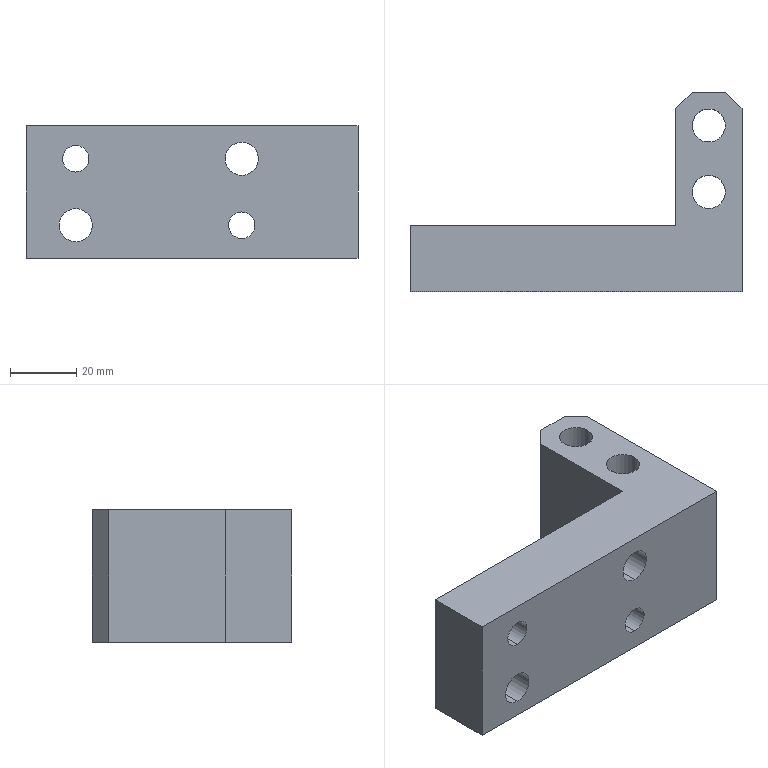Part | STEP file | HXGR200008-05-08 | 1 solid | 22 faces | box 100 x 60 x 40 mm | volume 99565 mm3 | cylinder 12 | plane 10 | commonest cylinder face diameters 10 x8 8 x4
STEP:
#1=CARTESIAN_POINT('',(-25.,0.,-14.));
#2=VERTEX_POINT('',#1);
#3=CARTESIAN_POINT('',(-25.,0.,-6.));
#4=VERTEX_POINT('',#3);
#5=CARTESIAN_POINT('',(-25.,0.,-10.));
#6=DIRECTION('',(0.,1.,0.));
#7=DIRECTION('',(0.,0.,1.));
#8=AXIS2_PLACEMENT_3D('',#5,#6,#7);
#9=CIRCLE('',#8,4.);
#10=EDGE_CURVE('',#2,#4,#9,.T.);
#11=ORIENTED_EDGE('',*,*,#10,.F.);
#12=CARTESIAN_POINT('',(-25.,20.,-14.));
#13=VERTEX_POINT('',#12);
#14=CARTESIAN_POINT('',(-25.,20.,-14.));
#15=DIRECTION('',(0.,1.,0.));
#16=VECTOR('',#15,1000.);
#17=LINE('',#14,#16);
#18=EDGE_CURVE('',#2,#13,#17,.T.);
#19=ORIENTED_EDGE('',*,*,#18,.T.);
#20=CARTESIAN_POINT('',(-25.,20.,-6.));
#21=VERTEX_POINT('',#20);
#22=CARTESIAN_POINT('',(-25.,20.,-10.));
#23=DIRECTION('',(0.,1.,0.));
#24=DIRECTION('',(0.,0.,1.));
#25=AXIS2_PLACEMENT_3D('',#22,#23,#24);
#26=CIRCLE('',#25,4.);
#27=EDGE_CURVE('',#13,#21,#26,.T.);
#28=ORIENTED_EDGE('',*,*,#27,.T.);
#29=CARTESIAN_POINT('',(-25.,20.,-6.));
#30=DIRECTION('',(0.,1.,0.));
#31=VECTOR('',#30,1000.);
#32=LINE('',#29,#31);
#33=EDGE_CURVE('',#4,#21,#32,.T.);
#34=ORIENTED_EDGE('',*,*,#33,.F.);
#35=EDGE_LOOP('',(#11,#19,#28,#34));
#36=FACE_OUTER_BOUND('',#35,.T.);
#37=CARTESIAN_POINT('',(-25.,20.,-10.));
#38=DIRECTION('',(0.,1.,0.));
#39=DIRECTION('',(0.,0.,1.));
#40=AXIS2_PLACEMENT_3D('',#37,#38,#39);
#41=CYLINDRICAL_SURFACE('',#40,4.);
#42=ADVANCED_FACE('',(#36),#41,.F.);
#43=CARTESIAN_POINT('',(-75.,0.,6.));
#44=VERTEX_POINT('',#43);
#45=CARTESIAN_POINT('',(-75.,0.,14.));
#46=VERTEX_POINT('',#45);
#47=CARTESIAN_POINT('',(-75.,0.,10.));
#48=DIRECTION('',(0.,1.,0.));
#49=DIRECTION('',(0.,0.,1.));
#50=AXIS2_PLACEMENT_3D('',#47,#48,#49);
#51=CIRCLE('',#50,4.);
#52=EDGE_CURVE('',#44,#46,#51,.T.);
#53=ORIENTED_EDGE('',*,*,#52,.F.);
#54=CARTESIAN_POINT('',(-75.,20.,6.));
#55=VERTEX_POINT('',#54);
#56=CARTESIAN_POINT('',(-75.,20.,6.));
#57=DIRECTION('',(0.,1.,0.));
#58=VECTOR('',#57,1000.);
#59=LINE('',#56,#58);
#60=EDGE_CURVE('',#44,#55,#59,.T.);
#61=ORIENTED_EDGE('',*,*,#60,.T.);
#62=CARTESIAN_POINT('',(-75.,20.,14.));
#63=VERTEX_POINT('',#62);
#64=CARTESIAN_POINT('',(-75.,20.,10.));
#65=DIRECTION('',(0.,1.,0.));
#66=DIRECTION('',(0.,0.,1.));
#67=AXIS2_PLACEMENT_3D('',#64,#65,#66);
#68=CIRCLE('',#67,4.);
#69=EDGE_CURVE('',#55,#63,#68,.T.);
#70=ORIENTED_EDGE('',*,*,#69,.T.);
#71=CARTESIAN_POINT('',(-75.,20.,14.));
#72=DIRECTION('',(0.,1.,0.));
#73=VECTOR('',#72,1000.);
#74=LINE('',#71,#73);
#75=EDGE_CURVE('',#46,#63,#74,.T.);
#76=ORIENTED_EDGE('',*,*,#75,.F.);
#77=EDGE_LOOP('',(#53,#61,#70,#76));
#78=FACE_OUTER_BOUND('',#77,.T.);
#79=CARTESIAN_POINT('',(-75.,20.,10.));
#80=DIRECTION('',(0.,1.,0.));
#81=DIRECTION('',(0.,0.,1.));
#82=AXIS2_PLACEMENT_3D('',#79,#80,#81);
#83=CYLINDRICAL_SURFACE('',#82,4.);
#84=ADVANCED_FACE('',(#78),#83,.F.);
#85=CARTESIAN_POINT('',(-75.,0.,-15.));
#86=VERTEX_POINT('',#85);
#87=CARTESIAN_POINT('',(-75.,0.,-5.));
#88=VERTEX_POINT('',#87);
#89=CARTESIAN_POINT('',(-75.,0.,-10.));
#90=DIRECTION('',(0.,1.,0.));
#91=DIRECTION('',(0.,0.,1.));
#92=AXIS2_PLACEMENT_3D('',#89,#90,#91);
#93=CIRCLE('',#92,5.);
#94=EDGE_CURVE('',#86,#88,#93,.T.);
#95=ORIENTED_EDGE('',*,*,#94,.F.);
#96=CARTESIAN_POINT('',(-75.,20.,-15.));
#97=VERTEX_POINT('',#96);
#98=CARTESIAN_POINT('',(-75.,20.,-15.));
#99=DIRECTION('',(0.,1.,0.));
#100=VECTOR('',#99,1000.);
#101=LINE('',#98,#100);
#102=EDGE_CURVE('',#86,#97,#101,.T.);
#103=ORIENTED_EDGE('',*,*,#102,.T.);
#104=CARTESIAN_POINT('',(-75.,20.,-5.));
#105=VERTEX_POINT('',#104);
#106=CARTESIAN_POINT('',(-75.,20.,-10.));
#107=DIRECTION('',(0.,1.,0.));
#108=DIRECTION('',(0.,0.,1.));
#109=AXIS2_PLACEMENT_3D('',#106,#107,#108);
#110=CIRCLE('',#109,5.);
#111=EDGE_CURVE('',#97,#105,#110,.T.);
#112=ORIENTED_EDGE('',*,*,#111,.T.);
#113=CARTESIAN_POINT('',(-75.,20.,-5.));
#114=DIRECTION('',(0.,1.,0.));
#115=VECTOR('',#114,1000.);
#116=LINE('',#113,#115);
#117=EDGE_CURVE('',#88,#105,#116,.T.);
#118=ORIENTED_EDGE('',*,*,#117,.F.);
#119=EDGE_LOOP('',(#95,#103,#112,#118));
#120=FACE_OUTER_BOUND('',#119,.T.);
#121=CARTESIAN_POINT('',(-75.,20.,-10.));
#122=DIRECTION('',(0.,1.,0.));
#123=DIRECTION('',(0.,0.,1.));
#124=AXIS2_PLACEMENT_3D('',#121,#122,#123);
#125=CYLINDRICAL_SURFACE('',#124,5.);
#126=ADVANCED_FACE('',(#120),#125,.F.);
#127=CARTESIAN_POINT('',(-25.,0.,5.));
#128=VERTEX_POINT('',#127);
#129=CARTESIAN_POINT('',(-25.,0.,15.));
#130=VERTEX_POINT('',#129);
#131=CARTESIAN_POINT('',(-25.,0.,10.));
#132=DIRECTION('',(0.,1.,0.));
#133=DIRECTION('',(0.,0.,1.));
#134=AXIS2_PLACEMENT_3D('',#131,#132,#133);
#135=CIRCLE('',#134,5.);
#136=EDGE_CURVE('',#128,#130,#135,.T.);
#137=ORIENTED_EDGE('',*,*,#136,.F.);
#138=CARTESIAN_POINT('',(-25.,20.,5.));
#139=VERTEX_POINT('',#138);
#140=CARTESIAN_POINT('',(-25.,20.,5.));
#141=DIRECTION('',(0.,1.,0.));
#142=VECTOR('',#141,1000.);
#143=LINE('',#140,#142);
#144=EDGE_CURVE('',#128,#139,#143,.T.);
#145=ORIENTED_EDGE('',*,*,#144,.T.);
#146=CARTESIAN_POINT('',(-25.,20.,15.));
#147=VERTEX_POINT('',#146);
#148=CARTESIAN_POINT('',(-25.,20.,10.));
#149=DIRECTION('',(0.,1.,0.));
#150=DIRECTION('',(0.,0.,1.));
#151=AXIS2_PLACEMENT_3D('',#148,#149,#150);
#152=CIRCLE('',#151,5.);
#153=EDGE_CURVE('',#139,#147,#152,.T.);
#154=ORIENTED_EDGE('',*,*,#153,.T.);
#155=CARTESIAN_POINT('',(-25.,20.,15.));
#156=DIRECTION('',(0.,1.,0.));
#157=VECTOR('',#156,1000.);
#158=LINE('',#155,#157);
#159=EDGE_CURVE('',#130,#147,#158,.T.);
#160=ORIENTED_EDGE('',*,*,#159,.F.);
#161=EDGE_LOOP('',(#137,#145,#154,#160));
#162=FACE_OUTER_BOUND('',#161,.T.);
#163=CARTESIAN_POINT('',(-25.,20.,10.));
#164=DIRECTION('',(0.,1.,0.));
#165=DIRECTION('',(0.,0.,1.));
#166=AXIS2_PLACEMENT_3D('',#163,#164,#165);
#167=CYLINDRICAL_SURFACE('',#166,5.);
#168=ADVANCED_FACE('',(#162),#167,.F.);
#169=CARTESIAN_POINT('',(-5.,50.,-20.));
#170=VERTEX_POINT('',#169);
#171=CARTESIAN_POINT('',(5.,50.,-20.));
#172=VERTEX_POINT('',#171);
#173=CARTESIAN_POINT('',(0.,50.,-20.));
#174=DIRECTION('',(0.,0.,1.));
#175=DIRECTION('',(1.,0.,0.));
#176=AXIS2_PLACEMENT_3D('',#173,#174,#175);
#177=CIRCLE('',#176,5.);
#178=EDGE_CURVE('',#170,#172,#177,.T.);
#179=ORIENTED_EDGE('',*,*,#178,.F.);
#180=CARTESIAN_POINT('',(-5.,50.,20.));
#181=VERTEX_POINT('',#180);
#182=CARTESIAN_POINT('',(-5.,50.,20.));
#183=DIRECTION('',(0.,0.,1.));
#184=VECTOR('',#183,1000.);
#185=LINE('',#182,#184);
#186=EDGE_CURVE('',#170,#181,#185,.T.);
#187=ORIENTED_EDGE('',*,*,#186,.T.);
#188=CARTESIAN_POINT('',(5.,50.,20.));
#189=VERTEX_POINT('',#188);
#190=CARTESIAN_POINT('',(0.,50.,20.));
#191=DIRECTION('',(0.,0.,1.));
#192=DIRECTION('',(1.,0.,0.));
#193=AXIS2_PLACEMENT_3D('',#190,#191,#192);
#194=CIRCLE('',#193,5.);
#195=EDGE_CURVE('',#181,#189,#194,.T.);
#196=ORIENTED_EDGE('',*,*,#195,.T.);
#197=CARTESIAN_POINT('',(5.,50.,20.));
#198=DIRECTION('',(0.,0.,1.));
#199=VECTOR('',#198,1000.);
#200=LINE('',#197,#199);
#201=EDGE_CURVE('',#172,#189,#200,.T.);
#202=ORIENTED_EDGE('',*,*,#201,.F.);
#203=EDGE_LOOP('',(#179,#187,#196,#202));
#204=FACE_OUTER_BOUND('',#203,.T.);
#205=CARTESIAN_POINT('',(0.,50.,20.));
#206=DIRECTION('',(0.,0.,1.));
#207=DIRECTION('',(1.,0.,0.));
#208=AXIS2_PLACEMENT_3D('',#205,#206,#207);
#209=CYLINDRICAL_SURFACE('',#208,5.);
#210=ADVANCED_FACE('',(#204),#209,.F.);
#211=CARTESIAN_POINT('',(-5.,30.,-20.));
#212=VERTEX_POINT('',#211);
#213=CARTESIAN_POINT('',(5.,30.,-20.));
#214=VERTEX_POINT('',#213);
#215=CARTESIAN_POINT('',(0.,30.,-20.));
#216=DIRECTION('',(0.,0.,1.));
#217=DIRECTION('',(1.,0.,0.));
#218=AXIS2_PLACEMENT_3D('',#215,#216,#217);
#219=CIRCLE('',#218,5.);
#220=EDGE_CURVE('',#212,#214,#219,.T.);
#221=ORIENTED_EDGE('',*,*,#220,.F.);
#222=CARTESIAN_POINT('',(-5.,30.,20.));
#223=VERTEX_POINT('',#222);
#224=CARTESIAN_POINT('',(-5.,30.,20.));
#225=DIRECTION('',(0.,0.,1.));
#226=VECTOR('',#225,1000.);
#227=LINE('',#224,#226);
#228=EDGE_CURVE('',#212,#223,#227,.T.);
#229=ORIENTED_EDGE('',*,*,#228,.T.);
#230=CARTESIAN_POINT('',(5.,30.,20.));
#231=VERTEX_POINT('',#230);
#232=CARTESIAN_POINT('',(0.,30.,20.));
#233=DIRECTION('',(0.,0.,1.));
#234=DIRECTION('',(1.,0.,0.));
#235=AXIS2_PLACEMENT_3D('',#232,#233,#234);
#236=CIRCLE('',#235,5.);
#237=EDGE_CURVE('',#223,#231,#236,.T.);
#238=ORIENTED_EDGE('',*,*,#237,.T.);
#239=CARTESIAN_POINT('',(5.,30.,20.));
#240=DIRECTION('',(0.,0.,1.));
#241=VECTOR('',#240,1000.);
#242=LINE('',#239,#241);
#243=EDGE_CURVE('',#214,#231,#242,.T.);
#244=ORIENTED_EDGE('',*,*,#243,.F.);
#245=EDGE_LOOP('',(#221,#229,#238,#244));
#246=FACE_OUTER_BOUND('',#245,.T.);
#247=CARTESIAN_POINT('',(0.,30.,20.));
#248=DIRECTION('',(0.,0.,1.));
#249=DIRECTION('',(1.,0.,0.));
#250=AXIS2_PLACEMENT_3D('',#247,#248,#249);
#251=CYLINDRICAL_SURFACE('',#250,5.);
#252=ADVANCED_FACE('',(#246),#251,.F.);
#253=CARTESIAN_POINT('',(10.,0.,-20.));
#254=VERTEX_POINT('',#253);
#255=CARTESIAN_POINT('',(10.,55.,-20.));
#256=VERTEX_POINT('',#255);
#257=CARTESIAN_POINT('',(10.,60.,-20.));
#258=DIRECTION('',(0.,1.,0.));
#259=VECTOR('',#258,1000.);
#260=LINE('',#257,#259);
#261=EDGE_CURVE('',#254,#256,#260,.T.);
#262=ORIENTED_EDGE('',*,*,#261,.T.);
#263=CARTESIAN_POINT('',(10.,55.,20.));
#264=VERTEX_POINT('',#263);
#265=CARTESIAN_POINT('',(10.,55.,20.));
#266=DIRECTION('',(0.,0.,1.));
#267=VECTOR('',#266,1000.);
#268=LINE('',#265,#267);
#269=EDGE_CURVE('',#256,#264,#268,.T.);
#270=ORIENTED_EDGE('',*,*,#269,.T.);
#271=CARTESIAN_POINT('',(10.,0.,20.));
#272=VERTEX_POINT('',#271);
#273=CARTESIAN_POINT('',(10.,60.,20.));
#274=DIRECTION('',(0.,1.,0.));
#275=VECTOR('',#274,1000.);
#276=LINE('',#273,#275);
#277=EDGE_CURVE('',#272,#264,#276,.T.);
#278=ORIENTED_EDGE('',*,*,#277,.F.);
#279=CARTESIAN_POINT('',(10.,0.,20.));
#280=DIRECTION('',(0.,0.,-1.));
#281=VECTOR('',#280,1000.);
#282=LINE('',#279,#281);
#283=EDGE_CURVE('',#272,#254,#282,.T.);
#284=ORIENTED_EDGE('',*,*,#283,.T.);
#285=EDGE_LOOP('',(#262,#270,#278,#284));
#286=FACE_OUTER_BOUND('',#285,.T.);
#287=CARTESIAN_POINT('',(10.,60.,20.));
#288=DIRECTION('',(-1.,0.,0.));
#289=DIRECTION('',(0.,-1.,0.));
#290=AXIS2_PLACEMENT_3D('',#287,#288,#289);
#291=PLANE('',#290);
#292=ADVANCED_FACE('',(#286),#291,.F.);
#293=CARTESIAN_POINT('',(5.,60.,20.));
#294=VERTEX_POINT('',#293);
#295=CARTESIAN_POINT('',(-5.,60.,20.));
#296=VERTEX_POINT('',#295);
#297=CARTESIAN_POINT('',(-10.,60.,20.));
#298=DIRECTION('',(-1.,0.,0.));
#299=VECTOR('',#298,1000.);
#300=LINE('',#297,#299);
#301=EDGE_CURVE('',#294,#296,#300,.T.);
#302=ORIENTED_EDGE('',*,*,#301,.F.);
#303=CARTESIAN_POINT('',(5.,60.,-20.));
#304=VERTEX_POINT('',#303);
#305=CARTESIAN_POINT('',(5.,60.,20.));
#306=DIRECTION('',(0.,0.,-1.));
#307=VECTOR('',#306,1000.);
#308=LINE('',#305,#307);
#309=EDGE_CURVE('',#294,#304,#308,.T.);
#310=ORIENTED_EDGE('',*,*,#309,.T.);
#311=CARTESIAN_POINT('',(-5.,60.,-20.));
#312=VERTEX_POINT('',#311);
#313=CARTESIAN_POINT('',(-10.,60.,-20.));
#314=DIRECTION('',(-1.,0.,0.));
#315=VECTOR('',#314,1000.);
#316=LINE('',#313,#315);
#317=EDGE_CURVE('',#304,#312,#316,.T.);
#318=ORIENTED_EDGE('',*,*,#317,.T.);
#319=CARTESIAN_POINT('',(-5.,60.,20.));
#320=DIRECTION('',(0.,0.,1.));
#321=VECTOR('',#320,1000.);
#322=LINE('',#319,#321);
#323=EDGE_CURVE('',#312,#296,#322,.T.);
#324=ORIENTED_EDGE('',*,*,#323,.T.);
#325=EDGE_LOOP('',(#302,#310,#318,#324));
#326=FACE_OUTER_BOUND('',#325,.T.);
#327=CARTESIAN_POINT('',(-10.,60.,20.));
#328=DIRECTION('',(0.,-1.,0.));
#329=DIRECTION('',(1.,0.,0.));
#330=AXIS2_PLACEMENT_3D('',#327,#328,#329);
#331=PLANE('',#330);
#332=ADVANCED_FACE('',(#326),#331,.F.);
#333=CARTESIAN_POINT('',(-10.,55.,20.));
#334=VERTEX_POINT('',#333);
#335=CARTESIAN_POINT('',(-10.,20.,20.));
#336=VERTEX_POINT('',#335);
#337=CARTESIAN_POINT('',(-10.,60.,20.));
#338=DIRECTION('',(0.,-1.,0.));
#339=VECTOR('',#338,1000.);
#340=LINE('',#337,#339);
#341=EDGE_CURVE('',#334,#336,#340,.T.);
#342=ORIENTED_EDGE('',*,*,#341,.F.);
#343=CARTESIAN_POINT('',(-10.,55.,-20.));
#344=VERTEX_POINT('',#343);
#345=CARTESIAN_POINT('',(-10.,55.,20.));
#346=DIRECTION('',(0.,0.,-1.));
#347=VECTOR('',#346,1000.);
#348=LINE('',#345,#347);
#349=EDGE_CURVE('',#334,#344,#348,.T.);
#350=ORIENTED_EDGE('',*,*,#349,.T.);
#351=CARTESIAN_POINT('',(-10.,20.,-20.));
#352=VERTEX_POINT('',#351);
#353=CARTESIAN_POINT('',(-10.,60.,-20.));
#354=DIRECTION('',(0.,-1.,0.));
#355=VECTOR('',#354,1000.);
#356=LINE('',#353,#355);
#357=EDGE_CURVE('',#344,#352,#356,.T.);
#358=ORIENTED_EDGE('',*,*,#357,.T.);
#359=CARTESIAN_POINT('',(-10.,20.,20.));
#360=DIRECTION('',(0.,0.,-1.));
#361=VECTOR('',#360,1000.);
#362=LINE('',#359,#361);
#363=EDGE_CURVE('',#336,#352,#362,.T.);
#364=ORIENTED_EDGE('',*,*,#363,.F.);
#365=EDGE_LOOP('',(#342,#350,#358,#364));
#366=FACE_OUTER_BOUND('',#365,.T.);
#367=CARTESIAN_POINT('',(-10.,60.,20.));
#368=DIRECTION('',(1.,0.,0.));
#369=DIRECTION('',(0.,1.,0.));
#370=AXIS2_PLACEMENT_3D('',#367,#368,#369);
#371=PLANE('',#370);
#372=ADVANCED_FACE('',(#366),#371,.F.);
#373=CARTESIAN_POINT('',(-25.,20.,-10.));
#374=DIRECTION('',(0.,1.,0.));
#375=DIRECTION('',(0.,0.,1.));
#376=AXIS2_PLACEMENT_3D('',#373,#374,#375);
#377=CIRCLE('',#376,4.);
#378=EDGE_CURVE('',#21,#13,#377,.T.);
#379=ORIENTED_EDGE('',*,*,#378,.F.);
#380=ORIENTED_EDGE('',*,*,#27,.F.);
#381=EDGE_LOOP('',(#379,#380));
#382=FACE_BOUND('',#381,.T.);
#383=CARTESIAN_POINT('',(-75.,20.,10.));
#384=DIRECTION('',(0.,1.,0.));
#385=DIRECTION('',(0.,0.,1.));
#386=AXIS2_PLACEMENT_3D('',#383,#384,#385);
#387=CIRCLE('',#386,4.);
#388=EDGE_CURVE('',#63,#55,#387,.T.);
#389=ORIENTED_EDGE('',*,*,#388,.F.);
#390=ORIENTED_EDGE('',*,*,#69,.F.);
#391=EDGE_LOOP('',(#389,#390));
#392=FACE_BOUND('',#391,.T.);
#393=CARTESIAN_POINT('',(-75.,20.,-10.));
#394=DIRECTION('',(0.,1.,0.));
#395=DIRECTION('',(0.,0.,1.));
#396=AXIS2_PLACEMENT_3D('',#393,#394,#395);
#397=CIRCLE('',#396,5.);
#398=EDGE_CURVE('',#105,#97,#397,.T.);
#399=ORIENTED_EDGE('',*,*,#398,.F.);
#400=ORIENTED_EDGE('',*,*,#111,.F.);
#401=EDGE_LOOP('',(#399,#400));
#402=FACE_BOUND('',#401,.T.);
#403=CARTESIAN_POINT('',(-25.,20.,10.));
#404=DIRECTION('',(0.,1.,0.));
#405=DIRECTION('',(0.,0.,1.));
#406=AXIS2_PLACEMENT_3D('',#403,#404,#405);
#407=CIRCLE('',#406,5.);
#408=EDGE_CURVE('',#147,#139,#407,.T.);
#409=ORIENTED_EDGE('',*,*,#408,.F.);
#410=ORIENTED_EDGE('',*,*,#153,.F.);
#411=EDGE_LOOP('',(#409,#410));
#412=FACE_BOUND('',#411,.T.);
#413=CARTESIAN_POINT('',(-90.,20.,-20.));
#414=VERTEX_POINT('',#413);
#415=CARTESIAN_POINT('',(-90.,20.,-20.));
#416=DIRECTION('',(-1.,0.,0.));
#417=VECTOR('',#416,1000.);
#418=LINE('',#415,#417);
#419=EDGE_CURVE('',#352,#414,#418,.T.);
#420=ORIENTED_EDGE('',*,*,#419,.T.);
#421=CARTESIAN_POINT('',(-90.,20.,20.));
#422=VERTEX_POINT('',#421);
#423=CARTESIAN_POINT('',(-90.,20.,20.));
#424=DIRECTION('',(0.,0.,-1.));
#425=VECTOR('',#424,1000.);
#426=LINE('',#423,#425);
#427=EDGE_CURVE('',#422,#414,#426,.T.);
#428=ORIENTED_EDGE('',*,*,#427,.F.);
#429=CARTESIAN_POINT('',(-90.,20.,20.));
#430=DIRECTION('',(-1.,0.,0.));
#431=VECTOR('',#430,1000.);
#432=LINE('',#429,#431);
#433=EDGE_CURVE('',#336,#422,#432,.T.);
#434=ORIENTED_EDGE('',*,*,#433,.F.);
#435=ORIENTED_EDGE('',*,*,#363,.T.);
#436=EDGE_LOOP('',(#420,#428,#434,#435));
#437=FACE_OUTER_BOUND('',#436,.T.);
#438=CARTESIAN_POINT('',(-90.,20.,20.));
#439=DIRECTION('',(0.,-1.,0.));
#440=DIRECTION('',(0.,0.,-1.));
#441=AXIS2_PLACEMENT_3D('',#438,#439,#440);
#442=PLANE('',#441);
#443=ADVANCED_FACE('',(#382,#392,#402,#412,#437),#442,.F.);
#444=CARTESIAN_POINT('',(-90.,0.,-20.));
#445=VERTEX_POINT('',#444);
#446=CARTESIAN_POINT('',(-90.,20.,-20.));
#447=DIRECTION('',(0.,-1.,0.));
#448=VECTOR('',#447,1000.);
#449=LINE('',#446,#448);
#450=EDGE_CURVE('',#414,#445,#449,.T.);
#451=ORIENTED_EDGE('',*,*,#450,.T.);
#452=CARTESIAN_POINT('',(-90.,0.,20.));
#453=VERTEX_POINT('',#452);
#454=CARTESIAN_POINT('',(-90.,0.,20.));
#455=DIRECTION('',(0.,0.,-1.));
#456=VECTOR('',#455,1000.);
#457=LINE('',#454,#456);
#458=EDGE_CURVE('',#453,#445,#457,.T.);
#459=ORIENTED_EDGE('',*,*,#458,.F.);
#460=CARTESIAN_POINT('',(-90.,20.,20.));
#461=DIRECTION('',(0.,-1.,0.));
#462=VECTOR('',#461,1000.);
#463=LINE('',#460,#462);
#464=EDGE_CURVE('',#422,#453,#463,.T.);
#465=ORIENTED_EDGE('',*,*,#464,.F.);
#466=ORIENTED_EDGE('',*,*,#427,.T.);
#467=EDGE_LOOP('',(#451,#459,#465,#466));
#468=FACE_OUTER_BOUND('',#467,.T.);
#469=CARTESIAN_POINT('',(-90.,20.,20.));
#470=DIRECTION('',(1.,0.,0.));
#471=DIRECTION('',(0.,1.,0.));
#472=AXIS2_PLACEMENT_3D('',#469,#470,#471);
#473=PLANE('',#472);
#474=ADVANCED_FACE('',(#468),#473,.F.);
#475=CARTESIAN_POINT('',(-25.,0.,-10.));
#476=DIRECTION('',(0.,1.,0.));
#477=DIRECTION('',(0.,0.,1.));
#478=AXIS2_PLACEMENT_3D('',#475,#476,#477);
#479=CIRCLE('',#478,4.);
#480=EDGE_CURVE('',#4,#2,#479,.T.);
#481=ORIENTED_EDGE('',*,*,#480,.T.);
#482=ORIENTED_EDGE('',*,*,#10,.T.);
#483=EDGE_LOOP('',(#481,#482));
#484=FACE_BOUND('',#483,.T.);
#485=CARTESIAN_POINT('',(-75.,0.,10.));
#486=DIRECTION('',(0.,1.,0.));
#487=DIRECTION('',(0.,0.,1.));
#488=AXIS2_PLACEMENT_3D('',#485,#486,#487);
#489=CIRCLE('',#488,4.);
#490=EDGE_CURVE('',#46,#44,#489,.T.);
#491=ORIENTED_EDGE('',*,*,#490,.T.);
#492=ORIENTED_EDGE('',*,*,#52,.T.);
#493=EDGE_LOOP('',(#491,#492));
#494=FACE_BOUND('',#493,.T.);
#495=CARTESIAN_POINT('',(-75.,0.,-10.));
#496=DIRECTION('',(0.,1.,0.));
#497=DIRECTION('',(0.,0.,1.));
#498=AXIS2_PLACEMENT_3D('',#495,#496,#497);
#499=CIRCLE('',#498,5.);
#500=EDGE_CURVE('',#88,#86,#499,.T.);
#501=ORIENTED_EDGE('',*,*,#500,.T.);
#502=ORIENTED_EDGE('',*,*,#94,.T.);
#503=EDGE_LOOP('',(#501,#502));
#504=FACE_BOUND('',#503,.T.);
#505=CARTESIAN_POINT('',(-25.,0.,10.));
#506=DIRECTION('',(0.,1.,0.));
#507=DIRECTION('',(0.,0.,1.));
#508=AXIS2_PLACEMENT_3D('',#505,#506,#507);
#509=CIRCLE('',#508,5.);
#510=EDGE_CURVE('',#130,#128,#509,.T.);
#511=ORIENTED_EDGE('',*,*,#510,.T.);
#512=ORIENTED_EDGE('',*,*,#136,.T.);
#513=EDGE_LOOP('',(#511,#512));
#514=FACE_BOUND('',#513,.T.);
#515=CARTESIAN_POINT('',(10.,0.,-20.));
#516=DIRECTION('',(1.,0.,0.));
#517=VECTOR('',#516,1000.);
#518=LINE('',#515,#517);
#519=EDGE_CURVE('',#445,#254,#518,.T.);
#520=ORIENTED_EDGE('',*,*,#519,.T.);
#521=ORIENTED_EDGE('',*,*,#283,.F.);
#522=CARTESIAN_POINT('',(10.,0.,20.));
#523=DIRECTION('',(1.,0.,0.));
#524=VECTOR('',#523,1000.);
#525=LINE('',#522,#524);
#526=EDGE_CURVE('',#453,#272,#525,.T.);
#527=ORIENTED_EDGE('',*,*,#526,.F.);
#528=ORIENTED_EDGE('',*,*,#458,.T.);
#529=EDGE_LOOP('',(#520,#521,#527,#528));
#530=FACE_OUTER_BOUND('',#529,.T.);
#531=CARTESIAN_POINT('',(10.,0.,20.));
#532=DIRECTION('',(0.,1.,0.));
#533=DIRECTION('',(-1.,0.,0.));
#534=AXIS2_PLACEMENT_3D('',#531,#532,#533);
#535=PLANE('',#534);
#536=ADVANCED_FACE('',(#484,#494,#504,#514,#530),#535,.F.);
#537=CARTESIAN_POINT('',(0.,50.,20.));
#538=DIRECTION('',(0.,0.,1.));
#539=DIRECTION('',(1.,0.,0.));
#540=AXIS2_PLACEMENT_3D('',#537,#538,#539);
#541=CIRCLE('',#540,5.);
#542=EDGE_CURVE('',#189,#181,#541,.T.);
#543=ORIENTED_EDGE('',*,*,#542,.F.);
#544=ORIENTED_EDGE('',*,*,#195,.F.);
#545=EDGE_LOOP('',(#543,#544));
#546=FACE_BOUND('',#545,.T.);
#547=CARTESIAN_POINT('',(0.,30.,20.));
#548=DIRECTION('',(0.,0.,1.));
#549=DIRECTION('',(1.,0.,0.));
#550=AXIS2_PLACEMENT_3D('',#547,#548,#549);
#551=CIRCLE('',#550,5.);
#552=EDGE_CURVE('',#231,#223,#551,.T.);
#553=ORIENTED_EDGE('',*,*,#552,.F.);
#554=ORIENTED_EDGE('',*,*,#237,.F.);
#555=EDGE_LOOP('',(#553,#554));
#556=FACE_BOUND('',#555,.T.);
#557=ORIENTED_EDGE('',*,*,#277,.T.);
#558=CARTESIAN_POINT('',(5.,60.,20.));
#559=DIRECTION('',(-0.7071,0.7071,0.));
#560=VECTOR('',#559,1000.);
#561=LINE('',#558,#560);
#562=EDGE_CURVE('',#264,#294,#561,.T.);
#563=ORIENTED_EDGE('',*,*,#562,.T.);
#564=ORIENTED_EDGE('',*,*,#301,.T.);
#565=CARTESIAN_POINT('',(-10.,55.,20.));
#566=DIRECTION('',(-0.7071,-0.7071,0.));
#567=VECTOR('',#566,1000.);
#568=LINE('',#565,#567);
#569=EDGE_CURVE('',#296,#334,#568,.T.);
#570=ORIENTED_EDGE('',*,*,#569,.T.);
#571=ORIENTED_EDGE('',*,*,#341,.T.);
#572=ORIENTED_EDGE('',*,*,#433,.T.);
#573=ORIENTED_EDGE('',*,*,#464,.T.);
#574=ORIENTED_EDGE('',*,*,#526,.T.);
#575=EDGE_LOOP('',(#557,#563,#564,#570,#571,#572,#573,#574));
#576=FACE_OUTER_BOUND('',#575,.T.);
#577=CARTESIAN_POINT('',(0.,0.,20.));
#578=DIRECTION('',(0.,0.,-1.));
#579=DIRECTION('',(-1.,0.,0.));
#580=AXIS2_PLACEMENT_3D('',#577,#578,#579);
#581=PLANE('',#580);
#582=ADVANCED_FACE('',(#546,#556,#576),#581,.F.);
#583=CARTESIAN_POINT('',(0.,50.,-20.));
#584=DIRECTION('',(0.,0.,1.));
#585=DIRECTION('',(1.,0.,0.));
#586=AXIS2_PLACEMENT_3D('',#583,#584,#585);
#587=CIRCLE('',#586,5.);
#588=EDGE_CURVE('',#172,#170,#587,.T.);
#589=ORIENTED_EDGE('',*,*,#588,.T.);
#590=ORIENTED_EDGE('',*,*,#178,.T.);
#591=EDGE_LOOP('',(#589,#590));
#592=FACE_BOUND('',#591,.T.);
#593=CARTESIAN_POINT('',(0.,30.,-20.));
#594=DIRECTION('',(0.,0.,1.));
#595=DIRECTION('',(1.,0.,0.));
#596=AXIS2_PLACEMENT_3D('',#593,#594,#595);
#597=CIRCLE('',#596,5.);
#598=EDGE_CURVE('',#214,#212,#597,.T.);
#599=ORIENTED_EDGE('',*,*,#598,.T.);
#600=ORIENTED_EDGE('',*,*,#220,.T.);
#601=EDGE_LOOP('',(#599,#600));
#602=FACE_BOUND('',#601,.T.);
#603=ORIENTED_EDGE('',*,*,#317,.F.);
#604=CARTESIAN_POINT('',(32.5,32.5,-20.));
#605=DIRECTION('',(0.7071,-0.7071,0.));
#606=VECTOR('',#605,1000.);
#607=LINE('',#604,#606);
#608=EDGE_CURVE('',#304,#256,#607,.T.);
#609=ORIENTED_EDGE('',*,*,#608,.T.);
#610=ORIENTED_EDGE('',*,*,#261,.F.);
#611=ORIENTED_EDGE('',*,*,#519,.F.);
#612=ORIENTED_EDGE('',*,*,#450,.F.);
#613=ORIENTED_EDGE('',*,*,#419,.F.);
#614=ORIENTED_EDGE('',*,*,#357,.F.);
#615=CARTESIAN_POINT('',(-32.5,32.5,-20.));
#616=DIRECTION('',(0.7071,0.7071,0.));
#617=VECTOR('',#616,1000.);
#618=LINE('',#615,#617);
#619=EDGE_CURVE('',#344,#312,#618,.T.);
#620=ORIENTED_EDGE('',*,*,#619,.T.);
#621=EDGE_LOOP('',(#603,#609,#610,#611,#612,#613,#614,#620));
#622=FACE_OUTER_BOUND('',#621,.T.);
#623=CARTESIAN_POINT('',(0.,0.,-20.));
#624=DIRECTION('',(0.,0.,-1.));
#625=DIRECTION('',(-1.,0.,0.));
#626=AXIS2_PLACEMENT_3D('',#623,#624,#625);
#627=PLANE('',#626);
#628=ADVANCED_FACE('',(#592,#602,#622),#627,.T.);
#629=ORIENTED_EDGE('',*,*,#228,.F.);
#630=ORIENTED_EDGE('',*,*,#598,.F.);
#631=ORIENTED_EDGE('',*,*,#243,.T.);
#632=ORIENTED_EDGE('',*,*,#552,.T.);
#633=EDGE_LOOP('',(#629,#630,#631,#632));
#634=FACE_OUTER_BOUND('',#633,.T.);
#635=CARTESIAN_POINT('',(0.,30.,20.));
#636=DIRECTION('',(0.,0.,1.));
#637=DIRECTION('',(1.,0.,0.));
#638=AXIS2_PLACEMENT_3D('',#635,#636,#637);
#639=CYLINDRICAL_SURFACE('',#638,5.);
#640=ADVANCED_FACE('',(#634),#639,.F.);
#641=ORIENTED_EDGE('',*,*,#186,.F.);
#642=ORIENTED_EDGE('',*,*,#588,.F.);
#643=ORIENTED_EDGE('',*,*,#201,.T.);
#644=ORIENTED_EDGE('',*,*,#542,.T.);
#645=EDGE_LOOP('',(#641,#642,#643,#644));
#646=FACE_OUTER_BOUND('',#645,.T.);
#647=CARTESIAN_POINT('',(0.,50.,20.));
#648=DIRECTION('',(0.,0.,1.));
#649=DIRECTION('',(1.,0.,0.));
#650=AXIS2_PLACEMENT_3D('',#647,#648,#649);
#651=CYLINDRICAL_SURFACE('',#650,5.);
#652=ADVANCED_FACE('',(#646),#651,.F.);
#653=ORIENTED_EDGE('',*,*,#562,.F.);
#654=ORIENTED_EDGE('',*,*,#269,.F.);
#655=ORIENTED_EDGE('',*,*,#608,.F.);
#656=ORIENTED_EDGE('',*,*,#309,.F.);
#657=EDGE_LOOP('',(#653,#654,#655,#656));
#658=FACE_OUTER_BOUND('',#657,.T.);
#659=CARTESIAN_POINT('',(5.,60.,20.));
#660=DIRECTION('',(-0.7071,-0.7071,0.));
#661=DIRECTION('',(0.,0.,-1.));
#662=AXIS2_PLACEMENT_3D('',#659,#660,#661);
#663=PLANE('',#662);
#664=ADVANCED_FACE('',(#658),#663,.F.);
#665=ORIENTED_EDGE('',*,*,#569,.F.);
#666=ORIENTED_EDGE('',*,*,#323,.F.);
#667=ORIENTED_EDGE('',*,*,#619,.F.);
#668=ORIENTED_EDGE('',*,*,#349,.F.);
#669=EDGE_LOOP('',(#665,#666,#667,#668));
#670=FACE_OUTER_BOUND('',#669,.T.);
#671=CARTESIAN_POINT('',(-10.,55.,20.));
#672=DIRECTION('',(0.7071,-0.7071,0.));
#673=DIRECTION('',(0.,0.,-1.));
#674=AXIS2_PLACEMENT_3D('',#671,#672,#673);
#675=PLANE('',#674);
#676=ADVANCED_FACE('',(#670),#675,.F.);
#677=ORIENTED_EDGE('',*,*,#144,.F.);
#678=ORIENTED_EDGE('',*,*,#510,.F.);
#679=ORIENTED_EDGE('',*,*,#159,.T.);
#680=ORIENTED_EDGE('',*,*,#408,.T.);
#681=EDGE_LOOP('',(#677,#678,#679,#680));
#682=FACE_OUTER_BOUND('',#681,.T.);
#683=CARTESIAN_POINT('',(-25.,20.,10.));
#684=DIRECTION('',(0.,1.,0.));
#685=DIRECTION('',(0.,0.,1.));
#686=AXIS2_PLACEMENT_3D('',#683,#684,#685);
#687=CYLINDRICAL_SURFACE('',#686,5.);
#688=ADVANCED_FACE('',(#682),#687,.F.);
#689=ORIENTED_EDGE('',*,*,#102,.F.);
#690=ORIENTED_EDGE('',*,*,#500,.F.);
#691=ORIENTED_EDGE('',*,*,#117,.T.);
#692=ORIENTED_EDGE('',*,*,#398,.T.);
#693=EDGE_LOOP('',(#689,#690,#691,#692));
#694=FACE_OUTER_BOUND('',#693,.T.);
#695=CARTESIAN_POINT('',(-75.,20.,-10.));
#696=DIRECTION('',(0.,1.,0.));
#697=DIRECTION('',(0.,0.,1.));
#698=AXIS2_PLACEMENT_3D('',#695,#696,#697);
#699=CYLINDRICAL_SURFACE('',#698,5.);
#700=ADVANCED_FACE('',(#694),#699,.F.);
#701=ORIENTED_EDGE('',*,*,#60,.F.);
#702=ORIENTED_EDGE('',*,*,#490,.F.);
#703=ORIENTED_EDGE('',*,*,#75,.T.);
#704=ORIENTED_EDGE('',*,*,#388,.T.);
#705=EDGE_LOOP('',(#701,#702,#703,#704));
#706=FACE_OUTER_BOUND('',#705,.T.);
#707=CARTESIAN_POINT('',(-75.,20.,10.));
#708=DIRECTION('',(0.,1.,0.));
#709=DIRECTION('',(0.,0.,1.));
#710=AXIS2_PLACEMENT_3D('',#707,#708,#709);
#711=CYLINDRICAL_SURFACE('',#710,4.);
#712=ADVANCED_FACE('',(#706),#711,.F.);
#713=ORIENTED_EDGE('',*,*,#18,.F.);
#714=ORIENTED_EDGE('',*,*,#480,.F.);
#715=ORIENTED_EDGE('',*,*,#33,.T.);
#716=ORIENTED_EDGE('',*,*,#378,.T.);
#717=EDGE_LOOP('',(#713,#714,#715,#716));
#718=FACE_OUTER_BOUND('',#717,.T.);
#719=CARTESIAN_POINT('',(-25.,20.,-10.));
#720=DIRECTION('',(0.,1.,0.));
#721=DIRECTION('',(0.,0.,1.));
#722=AXIS2_PLACEMENT_3D('',#719,#720,#721);
#723=CYLINDRICAL_SURFACE('',#722,4.);
#724=ADVANCED_FACE('',(#718),#723,.F.);
#725=CLOSED_SHELL('',(#42,#84,#126,#168,#210,#252,#292,#332,#372,#443,#474,#536,#582,#628,#640,#652,#664,#676,#688,#700,#712,#724));
#726=MANIFOLD_SOLID_BREP('',#725);
#727=CARTESIAN_POINT('',(0.,0.,0.));
#728=DIRECTION('',(0.,0.,1.));
#729=DIRECTION('',(1.,0.,0.));
#730=AXIS2_PLACEMENT_3D('',#727,#728,#729);
#731=(LENGTH_UNIT()NAMED_UNIT(*)SI_UNIT(.MILLI.,.METRE.));
#732=UNCERTAINTY_MEASURE_WITH_UNIT(LENGTH_MEASURE(0.00001),#731,'','');
#733=(NAMED_UNIT(*)PLANE_ANGLE_UNIT()SI_UNIT($,.RADIAN.));
#734=(NAMED_UNIT(*)SI_UNIT($,.STERADIAN.)SOLID_ANGLE_UNIT());
#735=(GEOMETRIC_REPRESENTATION_CONTEXT(3)GLOBAL_UNCERTAINTY_ASSIGNED_CONTEXT((#732))GLOBAL_UNIT_ASSIGNED_CONTEXT((#731,#733,#734))REPRESENTATION_CONTEXT('',''));
#736=ADVANCED_BREP_SHAPE_REPRESENTATION('',(#726,#730),#735);